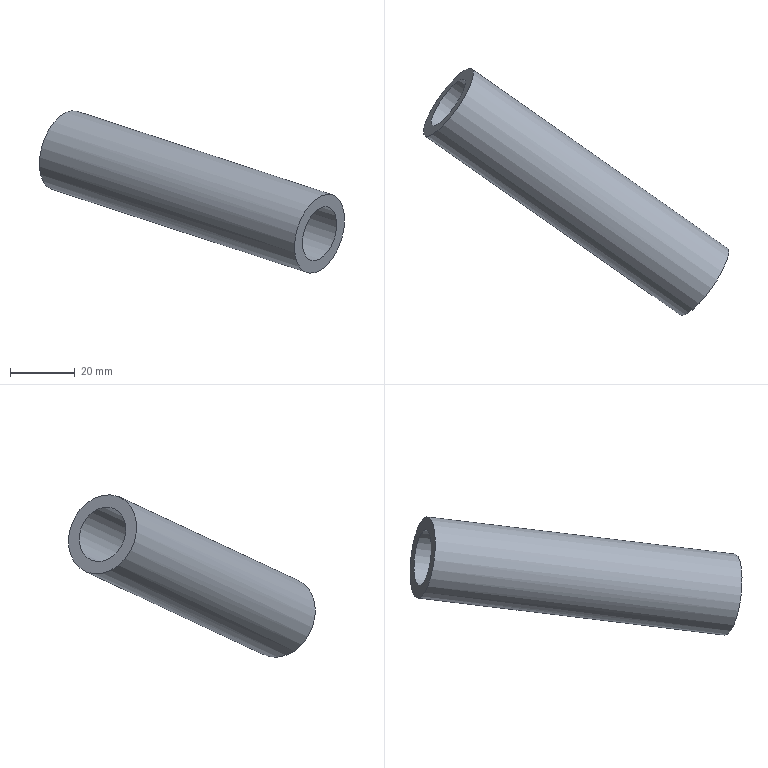Part | NX | features solid 2 | 1 solid | 4 faces | box 94.656 x 76.549 x 50.416 mm | volume 26892 mm3 | plane 2 | cylinder 2 | commonest cylinder face diameters 17.4 x1 25.4 x1
STEP:
#1=CARTESIAN_POINT('',(-125.95,665.398,3.857));
#2=VERTEX_POINT('',#1);
#3=CARTESIAN_POINT('',(-118.666,675.801,3.857));
#4=DIRECTION('',(-0.7912,0.554,0.2588));
#5=DIRECTION('',(-0.5736,-0.8192,0.));
#6=AXIS2_PLACEMENT_3D('',#3,#4,#5);
#7=CIRCLE('',#6,12.7);
#8=EDGE_CURVE('',#2,#2,#7,.F.);
#9=ORIENTED_EDGE('',*,*,#8,.T.);
#10=EDGE_LOOP('',(#9));
#11=FACE_BOUND('',#10,.T.);
#12=CARTESIAN_POINT('',(-123.656,668.674,3.857));
#13=VERTEX_POINT('',#12);
#14=CARTESIAN_POINT('',(-118.666,675.801,3.857));
#15=DIRECTION('',(-0.7912,0.554,0.2588));
#16=DIRECTION('',(-0.5736,-0.8192,0.));
#17=AXIS2_PLACEMENT_3D('',#14,#15,#16);
#18=CIRCLE('',#17,8.7);
#19=EDGE_CURVE('',#13,#13,#18,.F.);
#20=ORIENTED_EDGE('',*,*,#19,.F.);
#21=EDGE_LOOP('',(#20));
#22=FACE_BOUND('',#21,.T.);
#23=CARTESIAN_POINT('',(-118.666,675.801,3.857));
#24=DIRECTION('',(0.7912,-0.554,-0.2588));
#25=DIRECTION('',(-0.2557,-0.6842,0.683));
#26=AXIS2_PLACEMENT_3D('',#23,#24,#25);
#27=PLANE('',#26);
#28=ADVANCED_FACE('',(#11,#22),#27,.T.);
#29=CARTESIAN_POINT('',(-201.037,722.515,38.413));
#30=VERTEX_POINT('',#29);
#31=CARTESIAN_POINT('',(-197.79,731.204,29.738));
#32=DIRECTION('',(-0.7912,0.554,0.2588));
#33=DIRECTION('',(-0.2557,-0.6842,0.683));
#34=AXIS2_PLACEMENT_3D('',#31,#32,#33);
#35=CIRCLE('',#34,12.7);
#36=EDGE_CURVE('',#30,#30,#35,.F.);
#37=ORIENTED_EDGE('',*,*,#36,.F.);
#38=EDGE_LOOP('',(#37));
#39=FACE_BOUND('',#38,.T.);
#40=CARTESIAN_POINT('',(-195.566,737.157,23.796));
#41=VERTEX_POINT('',#40);
#42=CARTESIAN_POINT('',(-197.79,731.204,29.738));
#43=DIRECTION('',(0.7912,-0.554,-0.2588));
#44=DIRECTION('',(0.2557,0.6842,-0.683));
#45=AXIS2_PLACEMENT_3D('',#42,#43,#44);
#46=CIRCLE('',#45,8.7);
#47=EDGE_CURVE('',#41,#41,#46,.T.);
#48=ORIENTED_EDGE('',*,*,#47,.T.);
#49=EDGE_LOOP('',(#48));
#50=FACE_BOUND('',#49,.T.);
#51=CARTESIAN_POINT('',(-197.79,731.204,29.738));
#52=DIRECTION('',(0.7912,-0.554,-0.2588));
#53=DIRECTION('',(-0.2557,-0.6842,0.683));
#54=AXIS2_PLACEMENT_3D('',#51,#52,#53);
#55=PLANE('',#54);
#56=ADVANCED_FACE('',(#39,#50),#55,.F.);
#57=ORIENTED_EDGE('',*,*,#8,.F.);
#58=EDGE_LOOP('',(#57));
#59=FACE_BOUND('',#58,.T.);
#60=ORIENTED_EDGE('',*,*,#36,.T.);
#61=EDGE_LOOP('',(#60));
#62=FACE_BOUND('',#61,.T.);
#63=CARTESIAN_POINT('',(-197.79,731.204,29.738));
#64=DIRECTION('',(0.7912,-0.554,-0.2588));
#65=DIRECTION('',(-0.2557,-0.6842,0.683));
#66=AXIS2_PLACEMENT_3D('',#63,#64,#65);
#67=CYLINDRICAL_SURFACE('',#66,12.7);
#68=ADVANCED_FACE('',(#59,#62),#67,.T.);
#69=ORIENTED_EDGE('',*,*,#19,.T.);
#70=EDGE_LOOP('',(#69));
#71=FACE_BOUND('',#70,.T.);
#72=ORIENTED_EDGE('',*,*,#47,.F.);
#73=EDGE_LOOP('',(#72));
#74=FACE_BOUND('',#73,.T.);
#75=CARTESIAN_POINT('',(-197.79,731.204,29.738));
#76=DIRECTION('',(0.7912,-0.554,-0.2588));
#77=DIRECTION('',(-0.2557,-0.6842,0.683));
#78=AXIS2_PLACEMENT_3D('',#75,#76,#77);
#79=CYLINDRICAL_SURFACE('',#78,8.7);
#80=ADVANCED_FACE('',(#71,#74),#79,.F.);
#81=CLOSED_SHELL('',(#28,#56,#68,#80));
#82=MANIFOLD_SOLID_BREP('',#81);
#83=(LENGTH_UNIT()NAMED_UNIT(*)SI_UNIT(.MILLI.,.METRE.));
#84=UNCERTAINTY_MEASURE_WITH_UNIT(LENGTH_MEASURE(0.00001),#83,'','');
#85=(NAMED_UNIT(*)PLANE_ANGLE_UNIT()SI_UNIT($,.RADIAN.));
#86=(NAMED_UNIT(*)SI_UNIT($,.STERADIAN.)SOLID_ANGLE_UNIT());
#87=(GEOMETRIC_REPRESENTATION_CONTEXT(3)GLOBAL_UNCERTAINTY_ASSIGNED_CONTEXT((#84))GLOBAL_UNIT_ASSIGNED_CONTEXT((#83,#85,#86))REPRESENTATION_CONTEXT('',''));
#88=ADVANCED_BREP_SHAPE_REPRESENTATION('',(#82),#87);